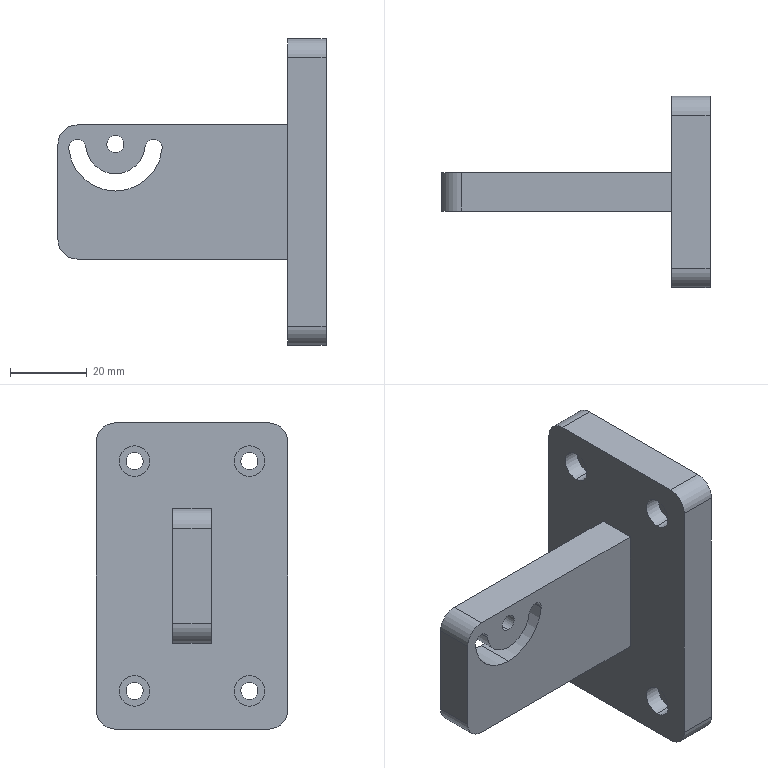Part | SolidWorks | features ICE 3, Extrusion 1, Fillet 1, HoleWzd 1 | 1 solid | 45 faces | box 70 x 50 x 80 mm | volume 57796 mm3 | cylinder 30 | plane 15 | commonest cylinder face diameters 4.5 x12 8 x8 10 x6 15.5 x2 24.5 x2
STEP:
#1=CARTESIAN_POINT('',(34.4,15.,26.));
#2=VERTEX_POINT('',#1);
#3=CARTESIAN_POINT('',(34.4,15.,34.));
#4=VERTEX_POINT('',#3);
#5=CARTESIAN_POINT('',(34.4,15.,30.));
#6=DIRECTION('',(-1.,0.,0.));
#7=DIRECTION('',(0.,0.,1.));
#8=AXIS2_PLACEMENT_3D('',#5,#6,#7);
#9=CIRCLE('',#8,4.);
#10=EDGE_CURVE('',#2,#4,#9,.T.);
#11=ORIENTED_EDGE('',*,*,#10,.F.);
#12=CARTESIAN_POINT('',(30.,15.,26.));
#13=VERTEX_POINT('',#12);
#14=CARTESIAN_POINT('',(30.,15.,26.));
#15=DIRECTION('',(-1.,0.,0.));
#16=VECTOR('',#15,1000.);
#17=LINE('',#14,#16);
#18=EDGE_CURVE('',#2,#13,#17,.T.);
#19=ORIENTED_EDGE('',*,*,#18,.T.);
#20=CARTESIAN_POINT('',(30.,15.,34.));
#21=VERTEX_POINT('',#20);
#22=CARTESIAN_POINT('',(30.,15.,30.));
#23=DIRECTION('',(-1.,0.,0.));
#24=DIRECTION('',(0.,0.,1.));
#25=AXIS2_PLACEMENT_3D('',#22,#23,#24);
#26=CIRCLE('',#25,4.);
#27=EDGE_CURVE('',#13,#21,#26,.T.);
#28=ORIENTED_EDGE('',*,*,#27,.T.);
#29=CARTESIAN_POINT('',(30.,15.,34.));
#30=DIRECTION('',(-1.,0.,0.));
#31=VECTOR('',#30,1000.);
#32=LINE('',#29,#31);
#33=EDGE_CURVE('',#4,#21,#32,.T.);
#34=ORIENTED_EDGE('',*,*,#33,.F.);
#35=EDGE_LOOP('',(#11,#19,#28,#34));
#36=FACE_OUTER_BOUND('',#35,.T.);
#37=CARTESIAN_POINT('',(30.,15.,30.));
#38=DIRECTION('',(-1.,0.,0.));
#39=DIRECTION('',(0.,0.,1.));
#40=AXIS2_PLACEMENT_3D('',#37,#38,#39);
#41=CYLINDRICAL_SURFACE('',#40,4.);
#42=ADVANCED_FACE('',(#36),#41,.F.);
#43=CARTESIAN_POINT('',(40.,15.,27.75));
#44=VERTEX_POINT('',#43);
#45=CARTESIAN_POINT('',(40.,15.,32.25));
#46=VERTEX_POINT('',#45);
#47=CARTESIAN_POINT('',(40.,15.,30.));
#48=DIRECTION('',(-1.,0.,0.));
#49=DIRECTION('',(0.,0.,1.));
#50=AXIS2_PLACEMENT_3D('',#47,#48,#49);
#51=CIRCLE('',#50,2.25);
#52=EDGE_CURVE('',#44,#46,#51,.T.);
#53=ORIENTED_EDGE('',*,*,#52,.F.);
#54=CARTESIAN_POINT('',(34.4,15.,27.75));
#55=VERTEX_POINT('',#54);
#56=CARTESIAN_POINT('',(30.,15.,27.75));
#57=DIRECTION('',(-1.,0.,0.));
#58=VECTOR('',#57,1000.);
#59=LINE('',#56,#58);
#60=EDGE_CURVE('',#44,#55,#59,.T.);
#61=ORIENTED_EDGE('',*,*,#60,.T.);
#62=CARTESIAN_POINT('',(34.4,15.,32.25));
#63=VERTEX_POINT('',#62);
#64=CARTESIAN_POINT('',(34.4,15.,30.));
#65=DIRECTION('',(-1.,0.,0.));
#66=DIRECTION('',(0.,0.,1.));
#67=AXIS2_PLACEMENT_3D('',#64,#65,#66);
#68=CIRCLE('',#67,2.25);
#69=EDGE_CURVE('',#55,#63,#68,.T.);
#70=ORIENTED_EDGE('',*,*,#69,.T.);
#71=CARTESIAN_POINT('',(30.,15.,32.25));
#72=DIRECTION('',(-1.,0.,0.));
#73=VECTOR('',#72,1000.);
#74=LINE('',#71,#73);
#75=EDGE_CURVE('',#46,#63,#74,.T.);
#76=ORIENTED_EDGE('',*,*,#75,.F.);
#77=EDGE_LOOP('',(#53,#61,#70,#76));
#78=FACE_OUTER_BOUND('',#77,.T.);
#79=CARTESIAN_POINT('',(30.,15.,30.));
#80=DIRECTION('',(-1.,0.,0.));
#81=DIRECTION('',(0.,0.,1.));
#82=AXIS2_PLACEMENT_3D('',#79,#80,#81);
#83=CYLINDRICAL_SURFACE('',#82,2.25);
#84=ADVANCED_FACE('',(#78),#83,.F.);
#85=CARTESIAN_POINT('',(34.4,15.,-34.));
#86=VERTEX_POINT('',#85);
#87=CARTESIAN_POINT('',(34.4,15.,-26.));
#88=VERTEX_POINT('',#87);
#89=CARTESIAN_POINT('',(34.4,15.,-30.));
#90=DIRECTION('',(-1.,0.,0.));
#91=DIRECTION('',(0.,0.,1.));
#92=AXIS2_PLACEMENT_3D('',#89,#90,#91);
#93=CIRCLE('',#92,4.);
#94=EDGE_CURVE('',#86,#88,#93,.T.);
#95=ORIENTED_EDGE('',*,*,#94,.F.);
#96=CARTESIAN_POINT('',(30.,15.,-34.));
#97=VERTEX_POINT('',#96);
#98=CARTESIAN_POINT('',(30.,15.,-34.));
#99=DIRECTION('',(-1.,0.,0.));
#100=VECTOR('',#99,1000.);
#101=LINE('',#98,#100);
#102=EDGE_CURVE('',#86,#97,#101,.T.);
#103=ORIENTED_EDGE('',*,*,#102,.T.);
#104=CARTESIAN_POINT('',(30.,15.,-26.));
#105=VERTEX_POINT('',#104);
#106=CARTESIAN_POINT('',(30.,15.,-30.));
#107=DIRECTION('',(-1.,0.,0.));
#108=DIRECTION('',(0.,0.,1.));
#109=AXIS2_PLACEMENT_3D('',#106,#107,#108);
#110=CIRCLE('',#109,4.);
#111=EDGE_CURVE('',#97,#105,#110,.T.);
#112=ORIENTED_EDGE('',*,*,#111,.T.);
#113=CARTESIAN_POINT('',(30.,15.,-26.));
#114=DIRECTION('',(-1.,0.,0.));
#115=VECTOR('',#114,1000.);
#116=LINE('',#113,#115);
#117=EDGE_CURVE('',#88,#105,#116,.T.);
#118=ORIENTED_EDGE('',*,*,#117,.F.);
#119=EDGE_LOOP('',(#95,#103,#112,#118));
#120=FACE_OUTER_BOUND('',#119,.T.);
#121=CARTESIAN_POINT('',(30.,15.,-30.));
#122=DIRECTION('',(-1.,0.,0.));
#123=DIRECTION('',(0.,0.,1.));
#124=AXIS2_PLACEMENT_3D('',#121,#122,#123);
#125=CYLINDRICAL_SURFACE('',#124,4.);
#126=ADVANCED_FACE('',(#120),#125,.F.);
#127=CARTESIAN_POINT('',(40.,15.,-32.25));
#128=VERTEX_POINT('',#127);
#129=CARTESIAN_POINT('',(40.,15.,-27.75));
#130=VERTEX_POINT('',#129);
#131=CARTESIAN_POINT('',(40.,15.,-30.));
#132=DIRECTION('',(-1.,0.,0.));
#133=DIRECTION('',(0.,0.,1.));
#134=AXIS2_PLACEMENT_3D('',#131,#132,#133);
#135=CIRCLE('',#134,2.25);
#136=EDGE_CURVE('',#128,#130,#135,.T.);
#137=ORIENTED_EDGE('',*,*,#136,.F.);
#138=CARTESIAN_POINT('',(34.4,15.,-32.25));
#139=VERTEX_POINT('',#138);
#140=CARTESIAN_POINT('',(30.,15.,-32.25));
#141=DIRECTION('',(-1.,0.,0.));
#142=VECTOR('',#141,1000.);
#143=LINE('',#140,#142);
#144=EDGE_CURVE('',#128,#139,#143,.T.);
#145=ORIENTED_EDGE('',*,*,#144,.T.);
#146=CARTESIAN_POINT('',(34.4,15.,-27.75));
#147=VERTEX_POINT('',#146);
#148=CARTESIAN_POINT('',(34.4,15.,-30.));
#149=DIRECTION('',(-1.,0.,0.));
#150=DIRECTION('',(0.,0.,1.));
#151=AXIS2_PLACEMENT_3D('',#148,#149,#150);
#152=CIRCLE('',#151,2.25);
#153=EDGE_CURVE('',#139,#147,#152,.T.);
#154=ORIENTED_EDGE('',*,*,#153,.T.);
#155=CARTESIAN_POINT('',(30.,15.,-27.75));
#156=DIRECTION('',(-1.,0.,0.));
#157=VECTOR('',#156,1000.);
#158=LINE('',#155,#157);
#159=EDGE_CURVE('',#130,#147,#158,.T.);
#160=ORIENTED_EDGE('',*,*,#159,.F.);
#161=EDGE_LOOP('',(#137,#145,#154,#160));
#162=FACE_OUTER_BOUND('',#161,.T.);
#163=CARTESIAN_POINT('',(30.,15.,-30.));
#164=DIRECTION('',(-1.,0.,0.));
#165=DIRECTION('',(0.,0.,1.));
#166=AXIS2_PLACEMENT_3D('',#163,#164,#165);
#167=CYLINDRICAL_SURFACE('',#166,2.25);
#168=ADVANCED_FACE('',(#162),#167,.F.);
#169=CARTESIAN_POINT('',(34.4,-15.,-34.));
#170=VERTEX_POINT('',#169);
#171=CARTESIAN_POINT('',(34.4,-15.,-26.));
#172=VERTEX_POINT('',#171);
#173=CARTESIAN_POINT('',(34.4,-15.,-30.));
#174=DIRECTION('',(-1.,0.,0.));
#175=DIRECTION('',(0.,0.,1.));
#176=AXIS2_PLACEMENT_3D('',#173,#174,#175);
#177=CIRCLE('',#176,4.);
#178=EDGE_CURVE('',#170,#172,#177,.T.);
#179=ORIENTED_EDGE('',*,*,#178,.F.);
#180=CARTESIAN_POINT('',(30.,-15.,-34.));
#181=VERTEX_POINT('',#180);
#182=CARTESIAN_POINT('',(30.,-15.,-34.));
#183=DIRECTION('',(-1.,0.,0.));
#184=VECTOR('',#183,1000.);
#185=LINE('',#182,#184);
#186=EDGE_CURVE('',#170,#181,#185,.T.);
#187=ORIENTED_EDGE('',*,*,#186,.T.);
#188=CARTESIAN_POINT('',(30.,-15.,-26.));
#189=VERTEX_POINT('',#188);
#190=CARTESIAN_POINT('',(30.,-15.,-30.));
#191=DIRECTION('',(-1.,0.,0.));
#192=DIRECTION('',(0.,0.,1.));
#193=AXIS2_PLACEMENT_3D('',#190,#191,#192);
#194=CIRCLE('',#193,4.);
#195=EDGE_CURVE('',#181,#189,#194,.T.);
#196=ORIENTED_EDGE('',*,*,#195,.T.);
#197=CARTESIAN_POINT('',(30.,-15.,-26.));
#198=DIRECTION('',(-1.,0.,0.));
#199=VECTOR('',#198,1000.);
#200=LINE('',#197,#199);
#201=EDGE_CURVE('',#172,#189,#200,.T.);
#202=ORIENTED_EDGE('',*,*,#201,.F.);
#203=EDGE_LOOP('',(#179,#187,#196,#202));
#204=FACE_OUTER_BOUND('',#203,.T.);
#205=CARTESIAN_POINT('',(30.,-15.,-30.));
#206=DIRECTION('',(-1.,0.,0.));
#207=DIRECTION('',(0.,0.,1.));
#208=AXIS2_PLACEMENT_3D('',#205,#206,#207);
#209=CYLINDRICAL_SURFACE('',#208,4.);
#210=ADVANCED_FACE('',(#204),#209,.F.);
#211=CARTESIAN_POINT('',(40.,-15.,-32.25));
#212=VERTEX_POINT('',#211);
#213=CARTESIAN_POINT('',(40.,-15.,-27.75));
#214=VERTEX_POINT('',#213);
#215=CARTESIAN_POINT('',(40.,-15.,-30.));
#216=DIRECTION('',(-1.,0.,0.));
#217=DIRECTION('',(0.,0.,1.));
#218=AXIS2_PLACEMENT_3D('',#215,#216,#217);
#219=CIRCLE('',#218,2.25);
#220=EDGE_CURVE('',#212,#214,#219,.T.);
#221=ORIENTED_EDGE('',*,*,#220,.F.);
#222=CARTESIAN_POINT('',(34.4,-15.,-32.25));
#223=VERTEX_POINT('',#222);
#224=CARTESIAN_POINT('',(30.,-15.,-32.25));
#225=DIRECTION('',(-1.,0.,0.));
#226=VECTOR('',#225,1000.);
#227=LINE('',#224,#226);
#228=EDGE_CURVE('',#212,#223,#227,.T.);
#229=ORIENTED_EDGE('',*,*,#228,.T.);
#230=CARTESIAN_POINT('',(34.4,-15.,-27.75));
#231=VERTEX_POINT('',#230);
#232=CARTESIAN_POINT('',(34.4,-15.,-30.));
#233=DIRECTION('',(-1.,0.,0.));
#234=DIRECTION('',(0.,0.,1.));
#235=AXIS2_PLACEMENT_3D('',#232,#233,#234);
#236=CIRCLE('',#235,2.25);
#237=EDGE_CURVE('',#223,#231,#236,.T.);
#238=ORIENTED_EDGE('',*,*,#237,.T.);
#239=CARTESIAN_POINT('',(30.,-15.,-27.75));
#240=DIRECTION('',(-1.,0.,0.));
#241=VECTOR('',#240,1000.);
#242=LINE('',#239,#241);
#243=EDGE_CURVE('',#214,#231,#242,.T.);
#244=ORIENTED_EDGE('',*,*,#243,.F.);
#245=EDGE_LOOP('',(#221,#229,#238,#244));
#246=FACE_OUTER_BOUND('',#245,.T.);
#247=CARTESIAN_POINT('',(30.,-15.,-30.));
#248=DIRECTION('',(-1.,0.,0.));
#249=DIRECTION('',(0.,0.,1.));
#250=AXIS2_PLACEMENT_3D('',#247,#248,#249);
#251=CYLINDRICAL_SURFACE('',#250,2.25);
#252=ADVANCED_FACE('',(#246),#251,.F.);
#253=CARTESIAN_POINT('',(34.4,-15.,26.));
#254=VERTEX_POINT('',#253);
#255=CARTESIAN_POINT('',(34.4,-15.,34.));
#256=VERTEX_POINT('',#255);
#257=CARTESIAN_POINT('',(34.4,-15.,30.));
#258=DIRECTION('',(-1.,0.,0.));
#259=DIRECTION('',(0.,0.,1.));
#260=AXIS2_PLACEMENT_3D('',#257,#258,#259);
#261=CIRCLE('',#260,4.);
#262=EDGE_CURVE('',#254,#256,#261,.T.);
#263=ORIENTED_EDGE('',*,*,#262,.F.);
#264=CARTESIAN_POINT('',(30.,-15.,26.));
#265=VERTEX_POINT('',#264);
#266=CARTESIAN_POINT('',(30.,-15.,26.));
#267=DIRECTION('',(-1.,0.,0.));
#268=VECTOR('',#267,1000.);
#269=LINE('',#266,#268);
#270=EDGE_CURVE('',#254,#265,#269,.T.);
#271=ORIENTED_EDGE('',*,*,#270,.T.);
#272=CARTESIAN_POINT('',(30.,-15.,34.));
#273=VERTEX_POINT('',#272);
#274=CARTESIAN_POINT('',(30.,-15.,30.));
#275=DIRECTION('',(-1.,0.,0.));
#276=DIRECTION('',(0.,0.,1.));
#277=AXIS2_PLACEMENT_3D('',#274,#275,#276);
#278=CIRCLE('',#277,4.);
#279=EDGE_CURVE('',#265,#273,#278,.T.);
#280=ORIENTED_EDGE('',*,*,#279,.T.);
#281=CARTESIAN_POINT('',(30.,-15.,34.));
#282=DIRECTION('',(-1.,0.,0.));
#283=VECTOR('',#282,1000.);
#284=LINE('',#281,#283);
#285=EDGE_CURVE('',#256,#273,#284,.T.);
#286=ORIENTED_EDGE('',*,*,#285,.F.);
#287=EDGE_LOOP('',(#263,#271,#280,#286));
#288=FACE_OUTER_BOUND('',#287,.T.);
#289=CARTESIAN_POINT('',(30.,-15.,30.));
#290=DIRECTION('',(-1.,0.,0.));
#291=DIRECTION('',(0.,0.,1.));
#292=AXIS2_PLACEMENT_3D('',#289,#290,#291);
#293=CYLINDRICAL_SURFACE('',#292,4.);
#294=ADVANCED_FACE('',(#288),#293,.F.);
#295=CARTESIAN_POINT('',(40.,-15.,27.75));
#296=VERTEX_POINT('',#295);
#297=CARTESIAN_POINT('',(40.,-15.,32.25));
#298=VERTEX_POINT('',#297);
#299=CARTESIAN_POINT('',(40.,-15.,30.));
#300=DIRECTION('',(-1.,0.,0.));
#301=DIRECTION('',(0.,0.,1.));
#302=AXIS2_PLACEMENT_3D('',#299,#300,#301);
#303=CIRCLE('',#302,2.25);
#304=EDGE_CURVE('',#296,#298,#303,.T.);
#305=ORIENTED_EDGE('',*,*,#304,.F.);
#306=CARTESIAN_POINT('',(34.4,-15.,27.75));
#307=VERTEX_POINT('',#306);
#308=CARTESIAN_POINT('',(30.,-15.,27.75));
#309=DIRECTION('',(-1.,0.,0.));
#310=VECTOR('',#309,1000.);
#311=LINE('',#308,#310);
#312=EDGE_CURVE('',#296,#307,#311,.T.);
#313=ORIENTED_EDGE('',*,*,#312,.T.);
#314=CARTESIAN_POINT('',(34.4,-15.,32.25));
#315=VERTEX_POINT('',#314);
#316=CARTESIAN_POINT('',(34.4,-15.,30.));
#317=DIRECTION('',(-1.,0.,0.));
#318=DIRECTION('',(0.,0.,1.));
#319=AXIS2_PLACEMENT_3D('',#316,#317,#318);
#320=CIRCLE('',#319,2.25);
#321=EDGE_CURVE('',#307,#315,#320,.T.);
#322=ORIENTED_EDGE('',*,*,#321,.T.);
#323=CARTESIAN_POINT('',(30.,-15.,32.25));
#324=DIRECTION('',(-1.,0.,0.));
#325=VECTOR('',#324,1000.);
#326=LINE('',#323,#325);
#327=EDGE_CURVE('',#298,#315,#326,.T.);
#328=ORIENTED_EDGE('',*,*,#327,.F.);
#329=EDGE_LOOP('',(#305,#313,#322,#328));
#330=FACE_OUTER_BOUND('',#329,.T.);
#331=CARTESIAN_POINT('',(30.,-15.,30.));
#332=DIRECTION('',(-1.,0.,0.));
#333=DIRECTION('',(0.,0.,1.));
#334=AXIS2_PLACEMENT_3D('',#331,#332,#333);
#335=CYLINDRICAL_SURFACE('',#334,2.25);
#336=ADVANCED_FACE('',(#330),#335,.F.);
#337=CARTESIAN_POINT('',(-15.,5.,4.75));
#338=VERTEX_POINT('',#337);
#339=CARTESIAN_POINT('',(-22.711,5.,11.725));
#340=VERTEX_POINT('',#339);
#341=CARTESIAN_POINT('',(-15.,5.,12.5));
#342=DIRECTION('',(0.,1.,0.));
#343=DIRECTION('',(0.,0.,-1.));
#344=AXIS2_PLACEMENT_3D('',#341,#342,#343);
#345=CIRCLE('',#344,7.75);
#346=EDGE_CURVE('',#338,#340,#345,.T.);
#347=ORIENTED_EDGE('',*,*,#346,.F.);
#348=CARTESIAN_POINT('',(-15.,-5.,4.75));
#349=VERTEX_POINT('',#348);
#350=CARTESIAN_POINT('',(-15.,5.,4.75));
#351=DIRECTION('',(0.,-1.,0.));
#352=VECTOR('',#351,1000.);
#353=LINE('',#350,#352);
#354=EDGE_CURVE('',#338,#349,#353,.T.);
#355=ORIENTED_EDGE('',*,*,#354,.T.);
#356=CARTESIAN_POINT('',(-22.711,-5.,11.725));
#357=VERTEX_POINT('',#356);
#358=CARTESIAN_POINT('',(-15.,-5.,12.5));
#359=DIRECTION('',(0.,1.,0.));
#360=DIRECTION('',(0.,0.,-1.));
#361=AXIS2_PLACEMENT_3D('',#358,#359,#360);
#362=CIRCLE('',#361,7.75);
#363=EDGE_CURVE('',#349,#357,#362,.T.);
#364=ORIENTED_EDGE('',*,*,#363,.T.);
#365=CARTESIAN_POINT('',(-22.711,5.,11.725));
#366=DIRECTION('',(0.,-1.,0.));
#367=VECTOR('',#366,1000.);
#368=LINE('',#365,#367);
#369=EDGE_CURVE('',#340,#357,#368,.T.);
#370=ORIENTED_EDGE('',*,*,#369,.F.);
#371=EDGE_LOOP('',(#347,#355,#364,#370));
#372=FACE_OUTER_BOUND('',#371,.T.);
#373=CARTESIAN_POINT('',(-15.,5.,12.5));
#374=DIRECTION('',(0.,-1.,0.));
#375=DIRECTION('',(0.,0.,-1.));
#376=AXIS2_PLACEMENT_3D('',#373,#374,#375);
#377=CYLINDRICAL_SURFACE('',#376,7.75);
#378=ADVANCED_FACE('',(#372),#377,.T.);
#379=CARTESIAN_POINT('',(-15.,5.,0.25));
#380=VERTEX_POINT('',#379);
#381=CARTESIAN_POINT('',(-2.811,5.,11.275));
#382=VERTEX_POINT('',#381);
#383=CARTESIAN_POINT('',(-15.,5.,12.5));
#384=DIRECTION('',(0.,-1.,0.));
#385=DIRECTION('',(0.,0.,-1.));
#386=AXIS2_PLACEMENT_3D('',#383,#384,#385);
#387=CIRCLE('',#386,12.25);
#388=EDGE_CURVE('',#380,#382,#387,.T.);
#389=ORIENTED_EDGE('',*,*,#388,.F.);
#390=CARTESIAN_POINT('',(-15.,-5.,0.25));
#391=VERTEX_POINT('',#390);
#392=CARTESIAN_POINT('',(-15.,5.,0.25));
#393=DIRECTION('',(0.,-1.,0.));
#394=VECTOR('',#393,1000.);
#395=LINE('',#392,#394);
#396=EDGE_CURVE('',#380,#391,#395,.T.);
#397=ORIENTED_EDGE('',*,*,#396,.T.);
#398=CARTESIAN_POINT('',(-2.811,-5.,11.275));
#399=VERTEX_POINT('',#398);
#400=CARTESIAN_POINT('',(-15.,-5.,12.5));
#401=DIRECTION('',(0.,-1.,0.));
#402=DIRECTION('',(0.,0.,-1.));
#403=AXIS2_PLACEMENT_3D('',#400,#401,#402);
#404=CIRCLE('',#403,12.25);
#405=EDGE_CURVE('',#391,#399,#404,.T.);
#406=ORIENTED_EDGE('',*,*,#405,.T.);
#407=CARTESIAN_POINT('',(-2.811,5.,11.275));
#408=DIRECTION('',(0.,-1.,0.));
#409=VECTOR('',#408,1000.);
#410=LINE('',#407,#409);
#411=EDGE_CURVE('',#382,#399,#410,.T.);
#412=ORIENTED_EDGE('',*,*,#411,.F.);
#413=EDGE_LOOP('',(#389,#397,#406,#412));
#414=FACE_OUTER_BOUND('',#413,.T.);
#415=CARTESIAN_POINT('',(-15.,5.,12.5));
#416=DIRECTION('',(0.,-1.,0.));
#417=DIRECTION('',(0.,0.,-1.));
#418=AXIS2_PLACEMENT_3D('',#415,#416,#417);
#419=CYLINDRICAL_SURFACE('',#418,12.25);
#420=ADVANCED_FACE('',(#414),#419,.F.);
#421=CARTESIAN_POINT('',(-15.,5.,14.75));
#422=VERTEX_POINT('',#421);
#423=CARTESIAN_POINT('',(-15.,5.,10.25));
#424=VERTEX_POINT('',#423);
#425=CARTESIAN_POINT('',(-15.,5.,12.5));
#426=DIRECTION('',(0.,-1.,0.));
#427=DIRECTION('',(0.,0.,-1.));
#428=AXIS2_PLACEMENT_3D('',#425,#426,#427);
#429=CIRCLE('',#428,2.25);
#430=EDGE_CURVE('',#422,#424,#429,.T.);
#431=ORIENTED_EDGE('',*,*,#430,.F.);
#432=CARTESIAN_POINT('',(-15.,-5.,14.75));
#433=VERTEX_POINT('',#432);
#434=CARTESIAN_POINT('',(-15.,5.,14.75));
#435=DIRECTION('',(0.,-1.,0.));
#436=VECTOR('',#435,1000.);
#437=LINE('',#434,#436);
#438=EDGE_CURVE('',#422,#433,#437,.T.);
#439=ORIENTED_EDGE('',*,*,#438,.T.);
#440=CARTESIAN_POINT('',(-15.,-5.,10.25));
#441=VERTEX_POINT('',#440);
#442=CARTESIAN_POINT('',(-15.,-5.,12.5));
#443=DIRECTION('',(0.,-1.,0.));
#444=DIRECTION('',(0.,0.,-1.));
#445=AXIS2_PLACEMENT_3D('',#442,#443,#444);
#446=CIRCLE('',#445,2.25);
#447=EDGE_CURVE('',#433,#441,#446,.T.);
#448=ORIENTED_EDGE('',*,*,#447,.T.);
#449=CARTESIAN_POINT('',(-15.,5.,10.25));
#450=DIRECTION('',(0.,-1.,0.));
#451=VECTOR('',#450,1000.);
#452=LINE('',#449,#451);
#453=EDGE_CURVE('',#424,#441,#452,.T.);
#454=ORIENTED_EDGE('',*,*,#453,.F.);
#455=EDGE_LOOP('',(#431,#439,#448,#454));
#456=FACE_OUTER_BOUND('',#455,.T.);
#457=CARTESIAN_POINT('',(-15.,5.,12.5));
#458=DIRECTION('',(0.,-1.,0.));
#459=DIRECTION('',(0.,0.,-1.));
#460=AXIS2_PLACEMENT_3D('',#457,#458,#459);
#461=CYLINDRICAL_SURFACE('',#460,2.25);
#462=ADVANCED_FACE('',(#456),#461,.F.);
#463=CARTESIAN_POINT('',(-15.,5.,12.5));
#464=DIRECTION('',(0.,-1.,0.));
#465=DIRECTION('',(0.,0.,-1.));
#466=AXIS2_PLACEMENT_3D('',#463,#464,#465);
#467=CIRCLE('',#466,2.25);
#468=EDGE_CURVE('',#424,#422,#467,.T.);
#469=ORIENTED_EDGE('',*,*,#468,.T.);
#470=ORIENTED_EDGE('',*,*,#430,.T.);
#471=EDGE_LOOP('',(#469,#470));
#472=FACE_BOUND('',#471,.T.);
#473=CARTESIAN_POINT('',(-30.,5.,-12.5));
#474=VERTEX_POINT('',#473);
#475=CARTESIAN_POINT('',(-30.,5.,12.5));
#476=VERTEX_POINT('',#475);
#477=CARTESIAN_POINT('',(-30.,5.,-17.5));
#478=DIRECTION('',(0.,0.,1.));
#479=VECTOR('',#478,1000.);
#480=LINE('',#477,#479);
#481=EDGE_CURVE('',#474,#476,#480,.T.);
#482=ORIENTED_EDGE('',*,*,#481,.T.);
#483=CARTESIAN_POINT('',(-25.,5.,17.5));
#484=VERTEX_POINT('',#483);
#485=CARTESIAN_POINT('',(-25.,5.,12.5));
#486=DIRECTION('',(0.,1.,0.));
#487=DIRECTION('',(0.,0.,1.));
#488=AXIS2_PLACEMENT_3D('',#485,#486,#487);
#489=CIRCLE('',#488,5.);
#490=EDGE_CURVE('',#476,#484,#489,.T.);
#491=ORIENTED_EDGE('',*,*,#490,.T.);
#492=CARTESIAN_POINT('',(30.,5.,17.5));
#493=VERTEX_POINT('',#492);
#494=CARTESIAN_POINT('',(-30.,5.,17.5));
#495=DIRECTION('',(1.,0.,0.));
#496=VECTOR('',#495,1000.);
#497=LINE('',#494,#496);
#498=EDGE_CURVE('',#484,#493,#497,.T.);
#499=ORIENTED_EDGE('',*,*,#498,.T.);
#500=CARTESIAN_POINT('',(30.,5.,-17.5));
#501=VERTEX_POINT('',#500);
#502=CARTESIAN_POINT('',(30.,5.,-17.5));
#503=DIRECTION('',(0.,0.,-1.));
#504=VECTOR('',#503,1000.);
#505=LINE('',#502,#504);
#506=EDGE_CURVE('',#493,#501,#505,.T.);
#507=ORIENTED_EDGE('',*,*,#506,.T.);
#508=CARTESIAN_POINT('',(-25.,5.,-17.5));
#509=VERTEX_POINT('',#508);
#510=CARTESIAN_POINT('',(-30.,5.,-17.5));
#511=DIRECTION('',(-1.,0.,0.));
#512=VECTOR('',#511,1000.);
#513=LINE('',#510,#512);
#514=EDGE_CURVE('',#501,#509,#513,.T.);
#515=ORIENTED_EDGE('',*,*,#514,.T.);
#516=CARTESIAN_POINT('',(-25.,5.,-12.5));
#517=DIRECTION('',(0.,1.,0.));
#518=DIRECTION('',(0.,0.,1.));
#519=AXIS2_PLACEMENT_3D('',#516,#517,#518);
#520=CIRCLE('',#519,5.);
#521=EDGE_CURVE('',#509,#474,#520,.T.);
#522=ORIENTED_EDGE('',*,*,#521,.T.);
#523=EDGE_LOOP('',(#482,#491,#499,#507,#515,#522));
#524=FACE_OUTER_BOUND('',#523,.T.);
#525=CARTESIAN_POINT('',(-7.289,5.,11.725));
#526=VERTEX_POINT('',#525);
#527=CARTESIAN_POINT('',(-5.05,5.,11.5));
#528=DIRECTION('',(0.,-1.,0.));
#529=DIRECTION('',(0.,0.,-1.));
#530=AXIS2_PLACEMENT_3D('',#527,#528,#529);
#531=CIRCLE('',#530,2.25);
#532=EDGE_CURVE('',#382,#526,#531,.T.);
#533=ORIENTED_EDGE('',*,*,#532,.T.);
#534=CARTESIAN_POINT('',(-15.,5.,12.5));
#535=DIRECTION('',(0.,1.,0.));
#536=DIRECTION('',(0.,0.,-1.));
#537=AXIS2_PLACEMENT_3D('',#534,#535,#536);
#538=CIRCLE('',#537,7.75);
#539=EDGE_CURVE('',#526,#338,#538,.T.);
#540=ORIENTED_EDGE('',*,*,#539,.T.);
#541=ORIENTED_EDGE('',*,*,#346,.T.);
#542=CARTESIAN_POINT('',(-27.189,5.,11.275));
#543=VERTEX_POINT('',#542);
#544=CARTESIAN_POINT('',(-24.95,5.,11.5));
#545=DIRECTION('',(0.,-1.,0.));
#546=DIRECTION('',(0.,0.,-1.));
#547=AXIS2_PLACEMENT_3D('',#544,#545,#546);
#548=CIRCLE('',#547,2.25);
#549=EDGE_CURVE('',#340,#543,#548,.T.);
#550=ORIENTED_EDGE('',*,*,#549,.T.);
#551=CARTESIAN_POINT('',(-15.,5.,12.5));
#552=DIRECTION('',(0.,-1.,0.));
#553=DIRECTION('',(0.,0.,-1.));
#554=AXIS2_PLACEMENT_3D('',#551,#552,#553);
#555=CIRCLE('',#554,12.25);
#556=EDGE_CURVE('',#543,#380,#555,.T.);
#557=ORIENTED_EDGE('',*,*,#556,.T.);
#558=ORIENTED_EDGE('',*,*,#388,.T.);
#559=EDGE_LOOP('',(#533,#540,#541,#550,#557,#558));
#560=FACE_BOUND('',#559,.T.);
#561=CARTESIAN_POINT('',(0.,5.,0.));
#562=DIRECTION('',(0.,1.,0.));
#563=DIRECTION('',(0.,0.,1.));
#564=AXIS2_PLACEMENT_3D('',#561,#562,#563);
#565=PLANE('',#564);
#566=ADVANCED_FACE('',(#472,#524,#560),#565,.T.);
#567=CARTESIAN_POINT('',(-15.,-5.,12.5));
#568=DIRECTION('',(0.,-1.,0.));
#569=DIRECTION('',(0.,0.,-1.));
#570=AXIS2_PLACEMENT_3D('',#567,#568,#569);
#571=CIRCLE('',#570,2.25);
#572=EDGE_CURVE('',#441,#433,#571,.T.);
#573=ORIENTED_EDGE('',*,*,#572,.F.);
#574=ORIENTED_EDGE('',*,*,#447,.F.);
#575=EDGE_LOOP('',(#573,#574));
#576=FACE_BOUND('',#575,.T.);
#577=CARTESIAN_POINT('',(-25.,-5.,17.5));
#578=VERTEX_POINT('',#577);
#579=CARTESIAN_POINT('',(30.,-5.,17.5));
#580=VERTEX_POINT('',#579);
#581=CARTESIAN_POINT('',(-30.,-5.,17.5));
#582=DIRECTION('',(1.,0.,0.));
#583=VECTOR('',#582,1000.);
#584=LINE('',#581,#583);
#585=EDGE_CURVE('',#578,#580,#584,.T.);
#586=ORIENTED_EDGE('',*,*,#585,.F.);
#587=CARTESIAN_POINT('',(-30.,-5.,12.5));
#588=VERTEX_POINT('',#587);
#589=CARTESIAN_POINT('',(-25.,-5.,12.5));
#590=DIRECTION('',(0.,-1.,0.));
#591=DIRECTION('',(0.,0.,1.));
#592=AXIS2_PLACEMENT_3D('',#589,#590,#591);
#593=CIRCLE('',#592,5.);
#594=EDGE_CURVE('',#578,#588,#593,.T.);
#595=ORIENTED_EDGE('',*,*,#594,.T.);
#596=CARTESIAN_POINT('',(-30.,-5.,-12.5));
#597=VERTEX_POINT('',#596);
#598=CARTESIAN_POINT('',(-30.,-5.,-17.5));
#599=DIRECTION('',(0.,0.,1.));
#600=VECTOR('',#599,1000.);
#601=LINE('',#598,#600);
#602=EDGE_CURVE('',#597,#588,#601,.T.);
#603=ORIENTED_EDGE('',*,*,#602,.F.);
#604=CARTESIAN_POINT('',(-25.,-5.,-17.5));
#605=VERTEX_POINT('',#604);
#606=CARTESIAN_POINT('',(-25.,-5.,-12.5));
#607=DIRECTION('',(0.,-1.,0.));
#608=DIRECTION('',(0.,0.,1.));
#609=AXIS2_PLACEMENT_3D('',#606,#607,#608);
#610=CIRCLE('',#609,5.);
#611=EDGE_CURVE('',#597,#605,#610,.T.);
#612=ORIENTED_EDGE('',*,*,#611,.T.);
#613=CARTESIAN_POINT('',(30.,-5.,-17.5));
#614=VERTEX_POINT('',#613);
#615=CARTESIAN_POINT('',(-30.,-5.,-17.5));
#616=DIRECTION('',(-1.,0.,0.));
#617=VECTOR('',#616,1000.);
#618=LINE('',#615,#617);
#619=EDGE_CURVE('',#614,#605,#618,.T.);
#620=ORIENTED_EDGE('',*,*,#619,.F.);
#621=CARTESIAN_POINT('',(30.,-5.,-17.5));
#622=DIRECTION('',(0.,0.,-1.));
#623=VECTOR('',#622,1000.);
#624=LINE('',#621,#623);
#625=EDGE_CURVE('',#580,#614,#624,.T.);
#626=ORIENTED_EDGE('',*,*,#625,.F.);
#627=EDGE_LOOP('',(#586,#595,#603,#612,#620,#626));
#628=FACE_OUTER_BOUND('',#627,.T.);
#629=CARTESIAN_POINT('',(-7.289,-5.,11.725));
#630=VERTEX_POINT('',#629);
#631=CARTESIAN_POINT('',(-15.,-5.,12.5));
#632=DIRECTION('',(0.,1.,0.));
#633=DIRECTION('',(0.,0.,-1.));
#634=AXIS2_PLACEMENT_3D('',#631,#632,#633);
#635=CIRCLE('',#634,7.75);
#636=EDGE_CURVE('',#630,#349,#635,.T.);
#637=ORIENTED_EDGE('',*,*,#636,.F.);
#638=CARTESIAN_POINT('',(-5.05,-5.,11.5));
#639=DIRECTION('',(0.,-1.,0.));
#640=DIRECTION('',(0.,0.,-1.));
#641=AXIS2_PLACEMENT_3D('',#638,#639,#640);
#642=CIRCLE('',#641,2.25);
#643=EDGE_CURVE('',#399,#630,#642,.T.);
#644=ORIENTED_EDGE('',*,*,#643,.F.);
#645=ORIENTED_EDGE('',*,*,#405,.F.);
#646=CARTESIAN_POINT('',(-27.189,-5.,11.275));
#647=VERTEX_POINT('',#646);
#648=CARTESIAN_POINT('',(-15.,-5.,12.5));
#649=DIRECTION('',(0.,-1.,0.));
#650=DIRECTION('',(0.,0.,-1.));
#651=AXIS2_PLACEMENT_3D('',#648,#649,#650);
#652=CIRCLE('',#651,12.25);
#653=EDGE_CURVE('',#647,#391,#652,.T.);
#654=ORIENTED_EDGE('',*,*,#653,.F.);
#655=CARTESIAN_POINT('',(-24.95,-5.,11.5));
#656=DIRECTION('',(0.,-1.,0.));
#657=DIRECTION('',(0.,0.,-1.));
#658=AXIS2_PLACEMENT_3D('',#655,#656,#657);
#659=CIRCLE('',#658,2.25);
#660=EDGE_CURVE('',#357,#647,#659,.T.);
#661=ORIENTED_EDGE('',*,*,#660,.F.);
#662=ORIENTED_EDGE('',*,*,#363,.F.);
#663=EDGE_LOOP('',(#637,#644,#645,#654,#661,#662));
#664=FACE_BOUND('',#663,.T.);
#665=CARTESIAN_POINT('',(0.,-5.,0.));
#666=DIRECTION('',(0.,1.,0.));
#667=DIRECTION('',(0.,0.,1.));
#668=AXIS2_PLACEMENT_3D('',#665,#666,#667);
#669=PLANE('',#668);
#670=ADVANCED_FACE('',(#576,#628,#664),#669,.F.);
#671=ORIENTED_EDGE('',*,*,#619,.T.);
#672=CARTESIAN_POINT('',(-25.,5.,-17.5));
#673=DIRECTION('',(0.,1.,0.));
#674=VECTOR('',#673,1000.);
#675=LINE('',#672,#674);
#676=EDGE_CURVE('',#605,#509,#675,.T.);
#677=ORIENTED_EDGE('',*,*,#676,.T.);
#678=ORIENTED_EDGE('',*,*,#514,.F.);
#679=CARTESIAN_POINT('',(30.,5.,-17.5));
#680=DIRECTION('',(0.,-1.,0.));
#681=VECTOR('',#680,1000.);
#682=LINE('',#679,#681);
#683=EDGE_CURVE('',#501,#614,#682,.T.);
#684=ORIENTED_EDGE('',*,*,#683,.T.);
#685=EDGE_LOOP('',(#671,#677,#678,#684));
#686=FACE_OUTER_BOUND('',#685,.T.);
#687=CARTESIAN_POINT('',(-30.,5.,-17.5));
#688=DIRECTION('',(0.,0.,1.));
#689=DIRECTION('',(1.,0.,0.));
#690=AXIS2_PLACEMENT_3D('',#687,#688,#689);
#691=PLANE('',#690);
#692=ADVANCED_FACE('',(#686),#691,.F.);
#693=ORIENTED_EDGE('',*,*,#602,.T.);
#694=CARTESIAN_POINT('',(-30.,5.,12.5));
#695=DIRECTION('',(0.,1.,0.));
#696=VECTOR('',#695,1000.);
#697=LINE('',#694,#696);
#698=EDGE_CURVE('',#588,#476,#697,.T.);
#699=ORIENTED_EDGE('',*,*,#698,.T.);
#700=ORIENTED_EDGE('',*,*,#481,.F.);
#701=CARTESIAN_POINT('',(-30.,5.,-12.5));
#702=DIRECTION('',(0.,-1.,0.));
#703=VECTOR('',#702,1000.);
#704=LINE('',#701,#703);
#705=EDGE_CURVE('',#474,#597,#704,.T.);
#706=ORIENTED_EDGE('',*,*,#705,.T.);
#707=EDGE_LOOP('',(#693,#699,#700,#706));
#708=FACE_OUTER_BOUND('',#707,.T.);
#709=CARTESIAN_POINT('',(-30.,5.,-17.5));
#710=DIRECTION('',(1.,0.,0.));
#711=DIRECTION('',(0.,0.,-1.));
#712=AXIS2_PLACEMENT_3D('',#709,#710,#711);
#713=PLANE('',#712);
#714=ADVANCED_FACE('',(#708),#713,.F.);
#715=ORIENTED_EDGE('',*,*,#498,.F.);
#716=CARTESIAN_POINT('',(-25.,5.,17.5));
#717=DIRECTION('',(0.,-1.,0.));
#718=VECTOR('',#717,1000.);
#719=LINE('',#716,#718);
#720=EDGE_CURVE('',#484,#578,#719,.T.);
#721=ORIENTED_EDGE('',*,*,#720,.T.);
#722=ORIENTED_EDGE('',*,*,#585,.T.);
#723=CARTESIAN_POINT('',(30.,5.,17.5));
#724=DIRECTION('',(0.,-1.,0.));
#725=VECTOR('',#724,1000.);
#726=LINE('',#723,#725);
#727=EDGE_CURVE('',#493,#580,#726,.T.);
#728=ORIENTED_EDGE('',*,*,#727,.F.);
#729=EDGE_LOOP('',(#715,#721,#722,#728));
#730=FACE_OUTER_BOUND('',#729,.T.);
#731=CARTESIAN_POINT('',(-30.,5.,17.5));
#732=DIRECTION('',(0.,0.,-1.));
#733=DIRECTION('',(-1.,0.,0.));
#734=AXIS2_PLACEMENT_3D('',#731,#732,#733);
#735=PLANE('',#734);
#736=ADVANCED_FACE('',(#730),#735,.F.);
#737=ORIENTED_EDGE('',*,*,#438,.F.);
#738=ORIENTED_EDGE('',*,*,#468,.F.);
#739=ORIENTED_EDGE('',*,*,#453,.T.);
#740=ORIENTED_EDGE('',*,*,#572,.T.);
#741=EDGE_LOOP('',(#737,#738,#739,#740));
#742=FACE_OUTER_BOUND('',#741,.T.);
#743=CARTESIAN_POINT('',(-15.,5.,12.5));
#744=DIRECTION('',(0.,-1.,0.));
#745=DIRECTION('',(0.,0.,-1.));
#746=AXIS2_PLACEMENT_3D('',#743,#744,#745);
#747=CYLINDRICAL_SURFACE('',#746,2.25);
#748=ADVANCED_FACE('',(#742),#747,.F.);
#749=ORIENTED_EDGE('',*,*,#396,.F.);
#750=ORIENTED_EDGE('',*,*,#556,.F.);
#751=CARTESIAN_POINT('',(-27.189,5.,11.275));
#752=DIRECTION('',(0.,-1.,0.));
#753=VECTOR('',#752,1000.);
#754=LINE('',#751,#753);
#755=EDGE_CURVE('',#543,#647,#754,.T.);
#756=ORIENTED_EDGE('',*,*,#755,.T.);
#757=ORIENTED_EDGE('',*,*,#653,.T.);
#758=EDGE_LOOP('',(#749,#750,#756,#757));
#759=FACE_OUTER_BOUND('',#758,.T.);
#760=CARTESIAN_POINT('',(-15.,5.,12.5));
#761=DIRECTION('',(0.,-1.,0.));
#762=DIRECTION('',(0.,0.,-1.));
#763=AXIS2_PLACEMENT_3D('',#760,#761,#762);
#764=CYLINDRICAL_SURFACE('',#763,12.25);
#765=ADVANCED_FACE('',(#759),#764,.F.);
#766=ORIENTED_EDGE('',*,*,#354,.F.);
#767=ORIENTED_EDGE('',*,*,#539,.F.);
#768=CARTESIAN_POINT('',(-7.289,5.,11.725));
#769=DIRECTION('',(0.,-1.,0.));
#770=VECTOR('',#769,1000.);
#771=LINE('',#768,#770);
#772=EDGE_CURVE('',#526,#630,#771,.T.);
#773=ORIENTED_EDGE('',*,*,#772,.T.);
#774=ORIENTED_EDGE('',*,*,#636,.T.);
#775=EDGE_LOOP('',(#766,#767,#773,#774));
#776=FACE_OUTER_BOUND('',#775,.T.);
#777=CARTESIAN_POINT('',(-15.,5.,12.5));
#778=DIRECTION('',(0.,-1.,0.));
#779=DIRECTION('',(0.,0.,-1.));
#780=AXIS2_PLACEMENT_3D('',#777,#778,#779);
#781=CYLINDRICAL_SURFACE('',#780,7.75);
#782=ADVANCED_FACE('',(#776),#781,.T.);
#783=ORIENTED_EDGE('',*,*,#643,.T.);
#784=ORIENTED_EDGE('',*,*,#772,.F.);
#785=ORIENTED_EDGE('',*,*,#532,.F.);
#786=ORIENTED_EDGE('',*,*,#411,.T.);
#787=EDGE_LOOP('',(#783,#784,#785,#786));
#788=FACE_OUTER_BOUND('',#787,.T.);
#789=CARTESIAN_POINT('',(-5.05,5.,11.5));
#790=DIRECTION('',(0.,-1.,0.));
#791=DIRECTION('',(0.,0.,-1.));
#792=AXIS2_PLACEMENT_3D('',#789,#790,#791);
#793=CYLINDRICAL_SURFACE('',#792,2.25);
#794=ADVANCED_FACE('',(#788),#793,.F.);
#795=ORIENTED_EDGE('',*,*,#660,.T.);
#796=ORIENTED_EDGE('',*,*,#755,.F.);
#797=ORIENTED_EDGE('',*,*,#549,.F.);
#798=ORIENTED_EDGE('',*,*,#369,.T.);
#799=EDGE_LOOP('',(#795,#796,#797,#798));
#800=FACE_OUTER_BOUND('',#799,.T.);
#801=CARTESIAN_POINT('',(-24.95,5.,11.5));
#802=DIRECTION('',(0.,-1.,0.));
#803=DIRECTION('',(0.,0.,-1.));
#804=AXIS2_PLACEMENT_3D('',#801,#802,#803);
#805=CYLINDRICAL_SURFACE('',#804,2.25);
#806=ADVANCED_FACE('',(#800),#805,.F.);
#807=CARTESIAN_POINT('',(30.,15.,30.));
#808=DIRECTION('',(-1.,0.,0.));
#809=DIRECTION('',(0.,0.,1.));
#810=AXIS2_PLACEMENT_3D('',#807,#808,#809);
#811=CIRCLE('',#810,4.);
#812=EDGE_CURVE('',#21,#13,#811,.T.);
#813=ORIENTED_EDGE('',*,*,#812,.F.);
#814=ORIENTED_EDGE('',*,*,#27,.F.);
#815=EDGE_LOOP('',(#813,#814));
#816=FACE_BOUND('',#815,.T.);
#817=CARTESIAN_POINT('',(30.,15.,-30.));
#818=DIRECTION('',(-1.,0.,0.));
#819=DIRECTION('',(0.,0.,1.));
#820=AXIS2_PLACEMENT_3D('',#817,#818,#819);
#821=CIRCLE('',#820,4.);
#822=EDGE_CURVE('',#105,#97,#821,.T.);
#823=ORIENTED_EDGE('',*,*,#822,.F.);
#824=ORIENTED_EDGE('',*,*,#111,.F.);
#825=EDGE_LOOP('',(#823,#824));
#826=FACE_BOUND('',#825,.T.);
#827=CARTESIAN_POINT('',(30.,-15.,-30.));
#828=DIRECTION('',(-1.,0.,0.));
#829=DIRECTION('',(0.,0.,1.));
#830=AXIS2_PLACEMENT_3D('',#827,#828,#829);
#831=CIRCLE('',#830,4.);
#832=EDGE_CURVE('',#189,#181,#831,.T.);
#833=ORIENTED_EDGE('',*,*,#832,.F.);
#834=ORIENTED_EDGE('',*,*,#195,.F.);
#835=EDGE_LOOP('',(#833,#834));
#836=FACE_BOUND('',#835,.T.);
#837=CARTESIAN_POINT('',(30.,-15.,30.));
#838=DIRECTION('',(-1.,0.,0.));
#839=DIRECTION('',(0.,0.,1.));
#840=AXIS2_PLACEMENT_3D('',#837,#838,#839);
#841=CIRCLE('',#840,4.);
#842=EDGE_CURVE('',#273,#265,#841,.T.);
#843=ORIENTED_EDGE('',*,*,#842,.F.);
#844=ORIENTED_EDGE('',*,*,#279,.F.);
#845=EDGE_LOOP('',(#843,#844));
#846=FACE_BOUND('',#845,.T.);
#847=CARTESIAN_POINT('',(30.,-25.,35.));
#848=VERTEX_POINT('',#847);
#849=CARTESIAN_POINT('',(30.,-25.,-35.));
#850=VERTEX_POINT('',#849);
#851=CARTESIAN_POINT('',(30.,-25.,40.));
#852=DIRECTION('',(0.,0.,-1.));
#853=VECTOR('',#852,1000.);
#854=LINE('',#851,#853);
#855=EDGE_CURVE('',#848,#850,#854,.T.);
#856=ORIENTED_EDGE('',*,*,#855,.F.);
#857=CARTESIAN_POINT('',(30.,-20.,40.));
#858=VERTEX_POINT('',#857);
#859=CARTESIAN_POINT('',(30.,-20.,35.));
#860=DIRECTION('',(-1.,0.,0.));
#861=DIRECTION('',(0.,0.,-1.));
#862=AXIS2_PLACEMENT_3D('',#859,#860,#861);
#863=CIRCLE('',#862,5.);
#864=EDGE_CURVE('',#848,#858,#863,.T.);
#865=ORIENTED_EDGE('',*,*,#864,.T.);
#866=CARTESIAN_POINT('',(30.,20.,40.));
#867=VERTEX_POINT('',#866);
#868=CARTESIAN_POINT('',(30.,25.,40.));
#869=DIRECTION('',(0.,-1.,0.));
#870=VECTOR('',#869,1000.);
#871=LINE('',#868,#870);
#872=EDGE_CURVE('',#867,#858,#871,.T.);
#873=ORIENTED_EDGE('',*,*,#872,.F.);
#874=CARTESIAN_POINT('',(30.,25.,35.));
#875=VERTEX_POINT('',#874);
#876=CARTESIAN_POINT('',(30.,20.,35.));
#877=DIRECTION('',(-1.,0.,0.));
#878=DIRECTION('',(0.,0.,-1.));
#879=AXIS2_PLACEMENT_3D('',#876,#877,#878);
#880=CIRCLE('',#879,5.);
#881=EDGE_CURVE('',#867,#875,#880,.T.);
#882=ORIENTED_EDGE('',*,*,#881,.T.);
#883=CARTESIAN_POINT('',(30.,25.,-35.));
#884=VERTEX_POINT('',#883);
#885=CARTESIAN_POINT('',(30.,25.,40.));
#886=DIRECTION('',(0.,0.,1.));
#887=VECTOR('',#886,1000.);
#888=LINE('',#885,#887);
#889=EDGE_CURVE('',#884,#875,#888,.T.);
#890=ORIENTED_EDGE('',*,*,#889,.F.);
#891=CARTESIAN_POINT('',(30.,20.,-40.));
#892=VERTEX_POINT('',#891);
#893=CARTESIAN_POINT('',(30.,20.,-35.));
#894=DIRECTION('',(-1.,0.,0.));
#895=DIRECTION('',(0.,0.,-1.));
#896=AXIS2_PLACEMENT_3D('',#893,#894,#895);
#897=CIRCLE('',#896,5.);
#898=EDGE_CURVE('',#884,#892,#897,.T.);
#899=ORIENTED_EDGE('',*,*,#898,.T.);
#900=CARTESIAN_POINT('',(30.,-20.,-40.));
#901=VERTEX_POINT('',#900);
#902=CARTESIAN_POINT('',(30.,25.,-40.));
#903=DIRECTION('',(0.,1.,0.));
#904=VECTOR('',#903,1000.);
#905=LINE('',#902,#904);
#906=EDGE_CURVE('',#901,#892,#905,.T.);
#907=ORIENTED_EDGE('',*,*,#906,.F.);
#908=CARTESIAN_POINT('',(30.,-20.,-35.));
#909=DIRECTION('',(-1.,0.,0.));
#910=DIRECTION('',(0.,0.,-1.));
#911=AXIS2_PLACEMENT_3D('',#908,#909,#910);
#912=CIRCLE('',#911,5.);
#913=EDGE_CURVE('',#901,#850,#912,.T.);
#914=ORIENTED_EDGE('',*,*,#913,.T.);
#915=EDGE_LOOP('',(#856,#865,#873,#882,#890,#899,#907,#914));
#916=FACE_OUTER_BOUND('',#915,.T.);
#917=ORIENTED_EDGE('',*,*,#727,.T.);
#918=ORIENTED_EDGE('',*,*,#625,.T.);
#919=ORIENTED_EDGE('',*,*,#683,.F.);
#920=ORIENTED_EDGE('',*,*,#506,.F.);
#921=EDGE_LOOP('',(#917,#918,#919,#920));
#922=FACE_BOUND('',#921,.T.);
#923=CARTESIAN_POINT('',(30.,0.,0.));
#924=DIRECTION('',(1.,0.,0.));
#925=DIRECTION('',(0.,0.,-1.));
#926=AXIS2_PLACEMENT_3D('',#923,#924,#925);
#927=PLANE('',#926);
#928=ADVANCED_FACE('',(#816,#826,#836,#846,#916,#922),#927,.F.);
#929=CARTESIAN_POINT('',(40.,-20.,-40.));
#930=VERTEX_POINT('',#929);
#931=CARTESIAN_POINT('',(40.,20.,-40.));
#932=VERTEX_POINT('',#931);
#933=CARTESIAN_POINT('',(40.,25.,-40.));
#934=DIRECTION('',(0.,1.,0.));
#935=VECTOR('',#934,1000.);
#936=LINE('',#933,#935);
#937=EDGE_CURVE('',#930,#932,#936,.T.);
#938=ORIENTED_EDGE('',*,*,#937,.F.);
#939=CARTESIAN_POINT('',(40.,-20.,-40.));
#940=DIRECTION('',(-1.,0.,0.));
#941=VECTOR('',#940,1000.);
#942=LINE('',#939,#941);
#943=EDGE_CURVE('',#930,#901,#942,.T.);
#944=ORIENTED_EDGE('',*,*,#943,.T.);
#945=ORIENTED_EDGE('',*,*,#906,.T.);
#946=CARTESIAN_POINT('',(40.,20.,-40.));
#947=DIRECTION('',(1.,0.,0.));
#948=VECTOR('',#947,1000.);
#949=LINE('',#946,#948);
#950=EDGE_CURVE('',#892,#932,#949,.T.);
#951=ORIENTED_EDGE('',*,*,#950,.T.);
#952=EDGE_LOOP('',(#938,#944,#945,#951));
#953=FACE_OUTER_BOUND('',#952,.T.);
#954=CARTESIAN_POINT('',(40.,25.,-40.));
#955=DIRECTION('',(0.,0.,1.));
#956=DIRECTION('',(1.,0.,0.));
#957=AXIS2_PLACEMENT_3D('',#954,#955,#956);
#958=PLANE('',#957);
#959=ADVANCED_FACE('',(#953),#958,.F.);
#960=ORIENTED_EDGE('',*,*,#889,.T.);
#961=CARTESIAN_POINT('',(40.,25.,35.));
#962=VERTEX_POINT('',#961);
#963=CARTESIAN_POINT('',(40.,25.,35.));
#964=DIRECTION('',(1.,0.,0.));
#965=VECTOR('',#964,1000.);
#966=LINE('',#963,#965);
#967=EDGE_CURVE('',#875,#962,#966,.T.);
#968=ORIENTED_EDGE('',*,*,#967,.T.);
#969=CARTESIAN_POINT('',(40.,25.,-35.));
#970=VERTEX_POINT('',#969);
#971=CARTESIAN_POINT('',(40.,25.,40.));
#972=DIRECTION('',(0.,0.,1.));
#973=VECTOR('',#972,1000.);
#974=LINE('',#971,#973);
#975=EDGE_CURVE('',#970,#962,#974,.T.);
#976=ORIENTED_EDGE('',*,*,#975,.F.);
#977=CARTESIAN_POINT('',(40.,25.,-35.));
#978=DIRECTION('',(-1.,0.,0.));
#979=VECTOR('',#978,1000.);
#980=LINE('',#977,#979);
#981=EDGE_CURVE('',#970,#884,#980,.T.);
#982=ORIENTED_EDGE('',*,*,#981,.T.);
#983=EDGE_LOOP('',(#960,#968,#976,#982));
#984=FACE_OUTER_BOUND('',#983,.T.);
#985=CARTESIAN_POINT('',(40.,25.,40.));
#986=DIRECTION('',(0.,-1.,0.));
#987=DIRECTION('',(0.,0.,-1.));
#988=AXIS2_PLACEMENT_3D('',#985,#986,#987);
#989=PLANE('',#988);
#990=ADVANCED_FACE('',(#984),#989,.F.);
#991=ORIENTED_EDGE('',*,*,#872,.T.);
#992=CARTESIAN_POINT('',(40.,-20.,40.));
#993=VERTEX_POINT('',#992);
#994=CARTESIAN_POINT('',(40.,-20.,40.));
#995=DIRECTION('',(1.,0.,0.));
#996=VECTOR('',#995,1000.);
#997=LINE('',#994,#996);
#998=EDGE_CURVE('',#858,#993,#997,.T.);
#999=ORIENTED_EDGE('',*,*,#998,.T.);
#1000=CARTESIAN_POINT('',(40.,20.,40.));
#1001=VERTEX_POINT('',#1000);
#1002=CARTESIAN_POINT('',(40.,25.,40.));
#1003=DIRECTION('',(0.,-1.,0.));
#1004=VECTOR('',#1003,1000.);
#1005=LINE('',#1002,#1004);
#1006=EDGE_CURVE('',#1001,#993,#1005,.T.);
#1007=ORIENTED_EDGE('',*,*,#1006,.F.);
#1008=CARTESIAN_POINT('',(40.,20.,40.));
#1009=DIRECTION('',(-1.,0.,0.));
#1010=VECTOR('',#1009,1000.);
#1011=LINE('',#1008,#1010);
#1012=EDGE_CURVE('',#1001,#867,#1011,.T.);
#1013=ORIENTED_EDGE('',*,*,#1012,.T.);
#1014=EDGE_LOOP('',(#991,#999,#1007,#1013));
#1015=FACE_OUTER_BOUND('',#1014,.T.);
#1016=CARTESIAN_POINT('',(40.,25.,40.));
#1017=DIRECTION('',(0.,0.,-1.));
#1018=DIRECTION('',(-1.,0.,0.));
#1019=AXIS2_PLACEMENT_3D('',#1016,#1017,#1018);
#1020=PLANE('',#1019);
#1021=ADVANCED_FACE('',(#1015),#1020,.F.);
#1022=CARTESIAN_POINT('',(40.,-25.,35.));
#1023=VERTEX_POINT('',#1022);
#1024=CARTESIAN_POINT('',(40.,-25.,-35.));
#1025=VERTEX_POINT('',#1024);
#1026=CARTESIAN_POINT('',(40.,-25.,40.));
#1027=DIRECTION('',(0.,0.,-1.));
#1028=VECTOR('',#1027,1000.);
#1029=LINE('',#1026,#1028);
#1030=EDGE_CURVE('',#1023,#1025,#1029,.T.);
#1031=ORIENTED_EDGE('',*,*,#1030,.F.);
#1032=CARTESIAN_POINT('',(40.,-25.,35.));
#1033=DIRECTION('',(-1.,0.,0.));
#1034=VECTOR('',#1033,1000.);
#1035=LINE('',#1032,#1034);
#1036=EDGE_CURVE('',#1023,#848,#1035,.T.);
#1037=ORIENTED_EDGE('',*,*,#1036,.T.);
#1038=ORIENTED_EDGE('',*,*,#855,.T.);
#1039=CARTESIAN_POINT('',(40.,-25.,-35.));
#1040=DIRECTION('',(1.,0.,0.));
#1041=VECTOR('',#1040,1000.);
#1042=LINE('',#1039,#1041);
#1043=EDGE_CURVE('',#850,#1025,#1042,.T.);
#1044=ORIENTED_EDGE('',*,*,#1043,.T.);
#1045=EDGE_LOOP('',(#1031,#1037,#1038,#1044));
#1046=FACE_OUTER_BOUND('',#1045,.T.);
#1047=CARTESIAN_POINT('',(40.,-25.,40.));
#1048=DIRECTION('',(0.,1.,0.));
#1049=DIRECTION('',(0.,0.,1.));
#1050=AXIS2_PLACEMENT_3D('',#1047,#1048,#1049);
#1051=PLANE('',#1050);
#1052=ADVANCED_FACE('',(#1046),#1051,.F.);
#1053=CARTESIAN_POINT('',(40.,15.,30.));
#1054=DIRECTION('',(-1.,0.,0.));
#1055=DIRECTION('',(0.,0.,1.));
#1056=AXIS2_PLACEMENT_3D('',#1053,#1054,#1055);
#1057=CIRCLE('',#1056,2.25);
#1058=EDGE_CURVE('',#46,#44,#1057,.T.);
#1059=ORIENTED_EDGE('',*,*,#1058,.T.);
#1060=ORIENTED_EDGE('',*,*,#52,.T.);
#1061=EDGE_LOOP('',(#1059,#1060));
#1062=FACE_BOUND('',#1061,.T.);
#1063=CARTESIAN_POINT('',(40.,15.,-30.));
#1064=DIRECTION('',(-1.,0.,0.));
#1065=DIRECTION('',(0.,0.,1.));
#1066=AXIS2_PLACEMENT_3D('',#1063,#1064,#1065);
#1067=CIRCLE('',#1066,2.25);
#1068=EDGE_CURVE('',#130,#128,#1067,.T.);
#1069=ORIENTED_EDGE('',*,*,#1068,.T.);
#1070=ORIENTED_EDGE('',*,*,#136,.T.);
#1071=EDGE_LOOP('',(#1069,#1070));
#1072=FACE_BOUND('',#1071,.T.);
#1073=CARTESIAN_POINT('',(40.,-15.,-30.));
#1074=DIRECTION('',(-1.,0.,0.));
#1075=DIRECTION('',(0.,0.,1.));
#1076=AXIS2_PLACEMENT_3D('',#1073,#1074,#1075);
#1077=CIRCLE('',#1076,2.25);
#1078=EDGE_CURVE('',#214,#212,#1077,.T.);
#1079=ORIENTED_EDGE('',*,*,#1078,.T.);
#1080=ORIENTED_EDGE('',*,*,#220,.T.);
#1081=EDGE_LOOP('',(#1079,#1080));
#1082=FACE_BOUND('',#1081,.T.);
#1083=CARTESIAN_POINT('',(40.,-15.,30.));
#1084=DIRECTION('',(-1.,0.,0.));
#1085=DIRECTION('',(0.,0.,1.));
#1086=AXIS2_PLACEMENT_3D('',#1083,#1084,#1085);
#1087=CIRCLE('',#1086,2.25);
#1088=EDGE_CURVE('',#298,#296,#1087,.T.);
#1089=ORIENTED_EDGE('',*,*,#1088,.T.);
#1090=ORIENTED_EDGE('',*,*,#304,.T.);
#1091=EDGE_LOOP('',(#1089,#1090));
#1092=FACE_BOUND('',#1091,.T.);
#1093=ORIENTED_EDGE('',*,*,#1006,.T.);
#1094=CARTESIAN_POINT('',(40.,-20.,35.));
#1095=DIRECTION('',(1.,0.,0.));
#1096=DIRECTION('',(0.,0.,-1.));
#1097=AXIS2_PLACEMENT_3D('',#1094,#1095,#1096);
#1098=CIRCLE('',#1097,5.);
#1099=EDGE_CURVE('',#993,#1023,#1098,.T.);
#1100=ORIENTED_EDGE('',*,*,#1099,.T.);
#1101=ORIENTED_EDGE('',*,*,#1030,.T.);
#1102=CARTESIAN_POINT('',(40.,-20.,-35.));
#1103=DIRECTION('',(1.,0.,0.));
#1104=DIRECTION('',(0.,0.,-1.));
#1105=AXIS2_PLACEMENT_3D('',#1102,#1103,#1104);
#1106=CIRCLE('',#1105,5.);
#1107=EDGE_CURVE('',#1025,#930,#1106,.T.);
#1108=ORIENTED_EDGE('',*,*,#1107,.T.);
#1109=ORIENTED_EDGE('',*,*,#937,.T.);
#1110=CARTESIAN_POINT('',(40.,20.,-35.));
#1111=DIRECTION('',(1.,0.,0.));
#1112=DIRECTION('',(0.,0.,-1.));
#1113=AXIS2_PLACEMENT_3D('',#1110,#1111,#1112);
#1114=CIRCLE('',#1113,5.);
#1115=EDGE_CURVE('',#932,#970,#1114,.T.);
#1116=ORIENTED_EDGE('',*,*,#1115,.T.);
#1117=ORIENTED_EDGE('',*,*,#975,.T.);
#1118=CARTESIAN_POINT('',(40.,20.,35.));
#1119=DIRECTION('',(1.,0.,0.));
#1120=DIRECTION('',(0.,0.,-1.));
#1121=AXIS2_PLACEMENT_3D('',#1118,#1119,#1120);
#1122=CIRCLE('',#1121,5.);
#1123=EDGE_CURVE('',#962,#1001,#1122,.T.);
#1124=ORIENTED_EDGE('',*,*,#1123,.T.);
#1125=EDGE_LOOP('',(#1093,#1100,#1101,#1108,#1109,#1116,#1117,#1124));
#1126=FACE_OUTER_BOUND('',#1125,.T.);
#1127=CARTESIAN_POINT('',(40.,0.,0.));
#1128=DIRECTION('',(1.,0.,0.));
#1129=DIRECTION('',(0.,0.,-1.));
#1130=AXIS2_PLACEMENT_3D('',#1127,#1128,#1129);
#1131=PLANE('',#1130);
#1132=ADVANCED_FACE('',(#1062,#1072,#1082,#1092,#1126),#1131,.T.);
#1133=ORIENTED_EDGE('',*,*,#312,.F.);
#1134=ORIENTED_EDGE('',*,*,#1088,.F.);
#1135=ORIENTED_EDGE('',*,*,#327,.T.);
#1136=CARTESIAN_POINT('',(34.4,-15.,30.));
#1137=DIRECTION('',(-1.,0.,0.));
#1138=DIRECTION('',(0.,0.,1.));
#1139=AXIS2_PLACEMENT_3D('',#1136,#1137,#1138);
#1140=CIRCLE('',#1139,2.25);
#1141=EDGE_CURVE('',#315,#307,#1140,.T.);
#1142=ORIENTED_EDGE('',*,*,#1141,.T.);
#1143=EDGE_LOOP('',(#1133,#1134,#1135,#1142));
#1144=FACE_OUTER_BOUND('',#1143,.T.);
#1145=CARTESIAN_POINT('',(30.,-15.,30.));
#1146=DIRECTION('',(-1.,0.,0.));
#1147=DIRECTION('',(0.,0.,1.));
#1148=AXIS2_PLACEMENT_3D('',#1145,#1146,#1147);
#1149=CYLINDRICAL_SURFACE('',#1148,2.25);
#1150=ADVANCED_FACE('',(#1144),#1149,.F.);
#1151=ORIENTED_EDGE('',*,*,#1141,.F.);
#1152=ORIENTED_EDGE('',*,*,#321,.F.);
#1153=EDGE_LOOP('',(#1151,#1152));
#1154=FACE_BOUND('',#1153,.T.);
#1155=CARTESIAN_POINT('',(34.4,-15.,30.));
#1156=DIRECTION('',(-1.,0.,0.));
#1157=DIRECTION('',(0.,0.,1.));
#1158=AXIS2_PLACEMENT_3D('',#1155,#1156,#1157);
#1159=CIRCLE('',#1158,4.);
#1160=EDGE_CURVE('',#256,#254,#1159,.T.);
#1161=ORIENTED_EDGE('',*,*,#1160,.T.);
#1162=ORIENTED_EDGE('',*,*,#262,.T.);
#1163=EDGE_LOOP('',(#1161,#1162));
#1164=FACE_OUTER_BOUND('',#1163,.T.);
#1165=CARTESIAN_POINT('',(34.4,-12.75,30.));
#1166=DIRECTION('',(1.,0.,0.));
#1167=DIRECTION('',(0.,0.,-1.));
#1168=AXIS2_PLACEMENT_3D('',#1165,#1166,#1167);
#1169=PLANE('',#1168);
#1170=ADVANCED_FACE('',(#1154,#1164),#1169,.F.);
#1171=ORIENTED_EDGE('',*,*,#270,.F.);
#1172=ORIENTED_EDGE('',*,*,#1160,.F.);
#1173=ORIENTED_EDGE('',*,*,#285,.T.);
#1174=ORIENTED_EDGE('',*,*,#842,.T.);
#1175=EDGE_LOOP('',(#1171,#1172,#1173,#1174));
#1176=FACE_OUTER_BOUND('',#1175,.T.);
#1177=CARTESIAN_POINT('',(30.,-15.,30.));
#1178=DIRECTION('',(-1.,0.,0.));
#1179=DIRECTION('',(0.,0.,1.));
#1180=AXIS2_PLACEMENT_3D('',#1177,#1178,#1179);
#1181=CYLINDRICAL_SURFACE('',#1180,4.);
#1182=ADVANCED_FACE('',(#1176),#1181,.F.);
#1183=ORIENTED_EDGE('',*,*,#228,.F.);
#1184=ORIENTED_EDGE('',*,*,#1078,.F.);
#1185=ORIENTED_EDGE('',*,*,#243,.T.);
#1186=CARTESIAN_POINT('',(34.4,-15.,-30.));
#1187=DIRECTION('',(-1.,0.,0.));
#1188=DIRECTION('',(0.,0.,1.));
#1189=AXIS2_PLACEMENT_3D('',#1186,#1187,#1188);
#1190=CIRCLE('',#1189,2.25);
#1191=EDGE_CURVE('',#231,#223,#1190,.T.);
#1192=ORIENTED_EDGE('',*,*,#1191,.T.);
#1193=EDGE_LOOP('',(#1183,#1184,#1185,#1192));
#1194=FACE_OUTER_BOUND('',#1193,.T.);
#1195=CARTESIAN_POINT('',(30.,-15.,-30.));
#1196=DIRECTION('',(-1.,0.,0.));
#1197=DIRECTION('',(0.,0.,1.));
#1198=AXIS2_PLACEMENT_3D('',#1195,#1196,#1197);
#1199=CYLINDRICAL_SURFACE('',#1198,2.25);
#1200=ADVANCED_FACE('',(#1194),#1199,.F.);
#1201=ORIENTED_EDGE('',*,*,#1191,.F.);
#1202=ORIENTED_EDGE('',*,*,#237,.F.);
#1203=EDGE_LOOP('',(#1201,#1202));
#1204=FACE_BOUND('',#1203,.T.);
#1205=CARTESIAN_POINT('',(34.4,-15.,-30.));
#1206=DIRECTION('',(-1.,0.,0.));
#1207=DIRECTION('',(0.,0.,1.));
#1208=AXIS2_PLACEMENT_3D('',#1205,#1206,#1207);
#1209=CIRCLE('',#1208,4.);
#1210=EDGE_CURVE('',#172,#170,#1209,.T.);
#1211=ORIENTED_EDGE('',*,*,#1210,.T.);
#1212=ORIENTED_EDGE('',*,*,#178,.T.);
#1213=EDGE_LOOP('',(#1211,#1212));
#1214=FACE_OUTER_BOUND('',#1213,.T.);
#1215=CARTESIAN_POINT('',(34.4,-12.75,-30.));
#1216=DIRECTION('',(1.,0.,0.));
#1217=DIRECTION('',(0.,0.,-1.));
#1218=AXIS2_PLACEMENT_3D('',#1215,#1216,#1217);
#1219=PLANE('',#1218);
#1220=ADVANCED_FACE('',(#1204,#1214),#1219,.F.);
#1221=ORIENTED_EDGE('',*,*,#186,.F.);
#1222=ORIENTED_EDGE('',*,*,#1210,.F.);
#1223=ORIENTED_EDGE('',*,*,#201,.T.);
#1224=ORIENTED_EDGE('',*,*,#832,.T.);
#1225=EDGE_LOOP('',(#1221,#1222,#1223,#1224));
#1226=FACE_OUTER_BOUND('',#1225,.T.);
#1227=CARTESIAN_POINT('',(30.,-15.,-30.));
#1228=DIRECTION('',(-1.,0.,0.));
#1229=DIRECTION('',(0.,0.,1.));
#1230=AXIS2_PLACEMENT_3D('',#1227,#1228,#1229);
#1231=CYLINDRICAL_SURFACE('',#1230,4.);
#1232=ADVANCED_FACE('',(#1226),#1231,.F.);
#1233=ORIENTED_EDGE('',*,*,#144,.F.);
#1234=ORIENTED_EDGE('',*,*,#1068,.F.);
#1235=ORIENTED_EDGE('',*,*,#159,.T.);
#1236=CARTESIAN_POINT('',(34.4,15.,-30.));
#1237=DIRECTION('',(-1.,0.,0.));
#1238=DIRECTION('',(0.,0.,1.));
#1239=AXIS2_PLACEMENT_3D('',#1236,#1237,#1238);
#1240=CIRCLE('',#1239,2.25);
#1241=EDGE_CURVE('',#147,#139,#1240,.T.);
#1242=ORIENTED_EDGE('',*,*,#1241,.T.);
#1243=EDGE_LOOP('',(#1233,#1234,#1235,#1242));
#1244=FACE_OUTER_BOUND('',#1243,.T.);
#1245=CARTESIAN_POINT('',(30.,15.,-30.));
#1246=DIRECTION('',(-1.,0.,0.));
#1247=DIRECTION('',(0.,0.,1.));
#1248=AXIS2_PLACEMENT_3D('',#1245,#1246,#1247);
#1249=CYLINDRICAL_SURFACE('',#1248,2.25);
#1250=ADVANCED_FACE('',(#1244),#1249,.F.);
#1251=ORIENTED_EDGE('',*,*,#1241,.F.);
#1252=ORIENTED_EDGE('',*,*,#153,.F.);
#1253=EDGE_LOOP('',(#1251,#1252));
#1254=FACE_BOUND('',#1253,.T.);
#1255=CARTESIAN_POINT('',(34.4,15.,-30.));
#1256=DIRECTION('',(-1.,0.,0.));
#1257=DIRECTION('',(0.,0.,1.));
#1258=AXIS2_PLACEMENT_3D('',#1255,#1256,#1257);
#1259=CIRCLE('',#1258,4.);
#1260=EDGE_CURVE('',#88,#86,#1259,.T.);
#1261=ORIENTED_EDGE('',*,*,#1260,.T.);
#1262=ORIENTED_EDGE('',*,*,#94,.T.);
#1263=EDGE_LOOP('',(#1261,#1262));
#1264=FACE_OUTER_BOUND('',#1263,.T.);
#1265=CARTESIAN_POINT('',(34.4,17.25,-30.));
#1266=DIRECTION('',(1.,0.,0.));
#1267=DIRECTION('',(0.,0.,-1.));
#1268=AXIS2_PLACEMENT_3D('',#1265,#1266,#1267);
#1269=PLANE('',#1268);
#1270=ADVANCED_FACE('',(#1254,#1264),#1269,.F.);
#1271=ORIENTED_EDGE('',*,*,#102,.F.);
#1272=ORIENTED_EDGE('',*,*,#1260,.F.);
#1273=ORIENTED_EDGE('',*,*,#117,.T.);
#1274=ORIENTED_EDGE('',*,*,#822,.T.);
#1275=EDGE_LOOP('',(#1271,#1272,#1273,#1274));
#1276=FACE_OUTER_BOUND('',#1275,.T.);
#1277=CARTESIAN_POINT('',(30.,15.,-30.));
#1278=DIRECTION('',(-1.,0.,0.));
#1279=DIRECTION('',(0.,0.,1.));
#1280=AXIS2_PLACEMENT_3D('',#1277,#1278,#1279);
#1281=CYLINDRICAL_SURFACE('',#1280,4.);
#1282=ADVANCED_FACE('',(#1276),#1281,.F.);
#1283=ORIENTED_EDGE('',*,*,#60,.F.);
#1284=ORIENTED_EDGE('',*,*,#1058,.F.);
#1285=ORIENTED_EDGE('',*,*,#75,.T.);
#1286=CARTESIAN_POINT('',(34.4,15.,30.));
#1287=DIRECTION('',(-1.,0.,0.));
#1288=DIRECTION('',(0.,0.,1.));
#1289=AXIS2_PLACEMENT_3D('',#1286,#1287,#1288);
#1290=CIRCLE('',#1289,2.25);
#1291=EDGE_CURVE('',#63,#55,#1290,.T.);
#1292=ORIENTED_EDGE('',*,*,#1291,.T.);
#1293=EDGE_LOOP('',(#1283,#1284,#1285,#1292));
#1294=FACE_OUTER_BOUND('',#1293,.T.);
#1295=CARTESIAN_POINT('',(30.,15.,30.));
#1296=DIRECTION('',(-1.,0.,0.));
#1297=DIRECTION('',(0.,0.,1.));
#1298=AXIS2_PLACEMENT_3D('',#1295,#1296,#1297);
#1299=CYLINDRICAL_SURFACE('',#1298,2.25);
#1300=ADVANCED_FACE('',(#1294),#1299,.F.);
#1301=ORIENTED_EDGE('',*,*,#1291,.F.);
#1302=ORIENTED_EDGE('',*,*,#69,.F.);
#1303=EDGE_LOOP('',(#1301,#1302));
#1304=FACE_BOUND('',#1303,.T.);
#1305=CARTESIAN_POINT('',(34.4,15.,30.));
#1306=DIRECTION('',(-1.,0.,0.));
#1307=DIRECTION('',(0.,0.,1.));
#1308=AXIS2_PLACEMENT_3D('',#1305,#1306,#1307);
#1309=CIRCLE('',#1308,4.);
#1310=EDGE_CURVE('',#4,#2,#1309,.T.);
#1311=ORIENTED_EDGE('',*,*,#1310,.T.);
#1312=ORIENTED_EDGE('',*,*,#10,.T.);
#1313=EDGE_LOOP('',(#1311,#1312));
#1314=FACE_OUTER_BOUND('',#1313,.T.);
#1315=CARTESIAN_POINT('',(34.4,17.25,30.));
#1316=DIRECTION('',(1.,0.,0.));
#1317=DIRECTION('',(0.,0.,-1.));
#1318=AXIS2_PLACEMENT_3D('',#1315,#1316,#1317);
#1319=PLANE('',#1318);
#1320=ADVANCED_FACE('',(#1304,#1314),#1319,.F.);
#1321=ORIENTED_EDGE('',*,*,#18,.F.);
#1322=ORIENTED_EDGE('',*,*,#1310,.F.);
#1323=ORIENTED_EDGE('',*,*,#33,.T.);
#1324=ORIENTED_EDGE('',*,*,#812,.T.);
#1325=EDGE_LOOP('',(#1321,#1322,#1323,#1324));
#1326=FACE_OUTER_BOUND('',#1325,.T.);
#1327=CARTESIAN_POINT('',(30.,15.,30.));
#1328=DIRECTION('',(-1.,0.,0.));
#1329=DIRECTION('',(0.,0.,1.));
#1330=AXIS2_PLACEMENT_3D('',#1327,#1328,#1329);
#1331=CYLINDRICAL_SURFACE('',#1330,4.);
#1332=ADVANCED_FACE('',(#1326),#1331,.F.);
#1333=ORIENTED_EDGE('',*,*,#1099,.F.);
#1334=ORIENTED_EDGE('',*,*,#998,.F.);
#1335=ORIENTED_EDGE('',*,*,#864,.F.);
#1336=ORIENTED_EDGE('',*,*,#1036,.F.);
#1337=EDGE_LOOP('',(#1333,#1334,#1335,#1336));
#1338=FACE_OUTER_BOUND('',#1337,.T.);
#1339=CARTESIAN_POINT('',(40.,-20.,35.));
#1340=DIRECTION('',(-1.,0.,0.));
#1341=DIRECTION('',(0.,0.,1.));
#1342=AXIS2_PLACEMENT_3D('',#1339,#1340,#1341);
#1343=CYLINDRICAL_SURFACE('',#1342,5.);
#1344=ADVANCED_FACE('',(#1338),#1343,.T.);
#1345=ORIENTED_EDGE('',*,*,#1123,.F.);
#1346=ORIENTED_EDGE('',*,*,#967,.F.);
#1347=ORIENTED_EDGE('',*,*,#881,.F.);
#1348=ORIENTED_EDGE('',*,*,#1012,.F.);
#1349=EDGE_LOOP('',(#1345,#1346,#1347,#1348));
#1350=FACE_OUTER_BOUND('',#1349,.T.);
#1351=CARTESIAN_POINT('',(40.,20.,35.));
#1352=DIRECTION('',(-1.,0.,0.));
#1353=DIRECTION('',(0.,0.,1.));
#1354=AXIS2_PLACEMENT_3D('',#1351,#1352,#1353);
#1355=CYLINDRICAL_SURFACE('',#1354,5.);
#1356=ADVANCED_FACE('',(#1350),#1355,.T.);
#1357=ORIENTED_EDGE('',*,*,#1107,.F.);
#1358=ORIENTED_EDGE('',*,*,#1043,.F.);
#1359=ORIENTED_EDGE('',*,*,#913,.F.);
#1360=ORIENTED_EDGE('',*,*,#943,.F.);
#1361=EDGE_LOOP('',(#1357,#1358,#1359,#1360));
#1362=FACE_OUTER_BOUND('',#1361,.T.);
#1363=CARTESIAN_POINT('',(40.,-20.,-35.));
#1364=DIRECTION('',(-1.,0.,0.));
#1365=DIRECTION('',(0.,0.,1.));
#1366=AXIS2_PLACEMENT_3D('',#1363,#1364,#1365);
#1367=CYLINDRICAL_SURFACE('',#1366,5.);
#1368=ADVANCED_FACE('',(#1362),#1367,.T.);
#1369=ORIENTED_EDGE('',*,*,#1115,.F.);
#1370=ORIENTED_EDGE('',*,*,#950,.F.);
#1371=ORIENTED_EDGE('',*,*,#898,.F.);
#1372=ORIENTED_EDGE('',*,*,#981,.F.);
#1373=EDGE_LOOP('',(#1369,#1370,#1371,#1372));
#1374=FACE_OUTER_BOUND('',#1373,.T.);
#1375=CARTESIAN_POINT('',(40.,20.,-35.));
#1376=DIRECTION('',(-1.,0.,0.));
#1377=DIRECTION('',(0.,0.,1.));
#1378=AXIS2_PLACEMENT_3D('',#1375,#1376,#1377);
#1379=CYLINDRICAL_SURFACE('',#1378,5.);
#1380=ADVANCED_FACE('',(#1374),#1379,.T.);
#1381=ORIENTED_EDGE('',*,*,#490,.F.);
#1382=ORIENTED_EDGE('',*,*,#698,.F.);
#1383=ORIENTED_EDGE('',*,*,#594,.F.);
#1384=ORIENTED_EDGE('',*,*,#720,.F.);
#1385=EDGE_LOOP('',(#1381,#1382,#1383,#1384));
#1386=FACE_OUTER_BOUND('',#1385,.T.);
#1387=CARTESIAN_POINT('',(-25.,5.,12.5));
#1388=DIRECTION('',(0.,-1.,0.));
#1389=DIRECTION('',(0.,0.,-1.));
#1390=AXIS2_PLACEMENT_3D('',#1387,#1388,#1389);
#1391=CYLINDRICAL_SURFACE('',#1390,5.);
#1392=ADVANCED_FACE('',(#1386),#1391,.T.);
#1393=ORIENTED_EDGE('',*,*,#521,.F.);
#1394=ORIENTED_EDGE('',*,*,#676,.F.);
#1395=ORIENTED_EDGE('',*,*,#611,.F.);
#1396=ORIENTED_EDGE('',*,*,#705,.F.);
#1397=EDGE_LOOP('',(#1393,#1394,#1395,#1396));
#1398=FACE_OUTER_BOUND('',#1397,.T.);
#1399=CARTESIAN_POINT('',(-25.,5.,-12.5));
#1400=DIRECTION('',(0.,-1.,0.));
#1401=DIRECTION('',(0.,0.,-1.));
#1402=AXIS2_PLACEMENT_3D('',#1399,#1400,#1401);
#1403=CYLINDRICAL_SURFACE('',#1402,5.);
#1404=ADVANCED_FACE('',(#1398),#1403,.T.);
#1405=CLOSED_SHELL('',(#42,#84,#126,#168,#210,#252,#294,#336,#378,#420,#462,#566,#670,#692,#714,#736,#748,#765,#782,#794,#806,#928,#959,#990,#1021,#1052,#1132,#1150,#1170,#1182,#1200,#1220,#1232,#1250,#1270,#1282,#1300,#1320,#1332,#1344,#1356,#1368,#1380,#1392,#1404));
#1406=MANIFOLD_SOLID_BREP('',#1405);
#1407=CARTESIAN_POINT('',(0.,0.,0.));
#1408=DIRECTION('',(0.,0.,1.));
#1409=DIRECTION('',(1.,0.,0.));
#1410=AXIS2_PLACEMENT_3D('',#1407,#1408,#1409);
#1411=(LENGTH_UNIT()NAMED_UNIT(*)SI_UNIT(.MILLI.,.METRE.));
#1412=UNCERTAINTY_MEASURE_WITH_UNIT(LENGTH_MEASURE(0.00001),#1411,'','');
#1413=(NAMED_UNIT(*)PLANE_ANGLE_UNIT()SI_UNIT($,.RADIAN.));
#1414=(NAMED_UNIT(*)SI_UNIT($,.STERADIAN.)SOLID_ANGLE_UNIT());
#1415=(GEOMETRIC_REPRESENTATION_CONTEXT(3)GLOBAL_UNCERTAINTY_ASSIGNED_CONTEXT((#1412))GLOBAL_UNIT_ASSIGNED_CONTEXT((#1411,#1413,#1414))REPRESENTATION_CONTEXT('',''));
#1416=ADVANCED_BREP_SHAPE_REPRESENTATION('',(#1406,#1410),#1415);